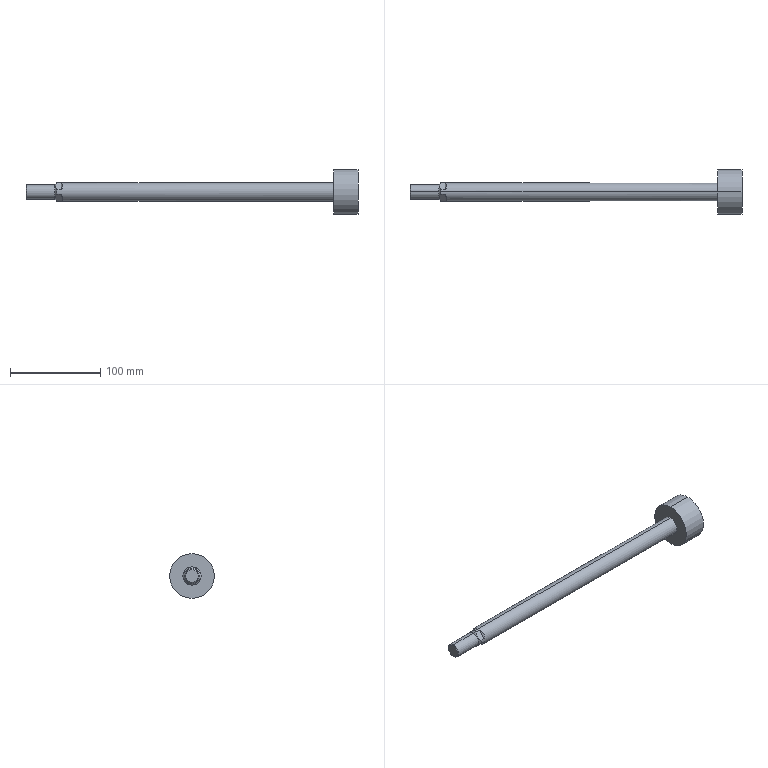Part | SolidWorks | features BaseBody 1 | 1 solid | 21 faces | box 367 x 49.5 x 49.5 mm | volume 154752 mm3 | plane 11 | cylinder 6 | cone 4 | commonest cylinder face diameters 16 x2 20 x2 49.5 x2
STEP:
#1=CARTESIAN_POINT('',(-57.,0.,-7.08));
#2=VERTEX_POINT('',#1);
#3=CARTESIAN_POINT('',(-57.,0.,7.08));
#4=VERTEX_POINT('',#3);
#5=CARTESIAN_POINT('',(-57.,0.,0.));
#6=DIRECTION('',(1.,0.,0.));
#7=DIRECTION('',(0.,0.,-1.));
#8=AXIS2_PLACEMENT_3D('',#5,#6,#7);
#9=CIRCLE('',#8,7.08);
#10=EDGE_CURVE('',#2,#4,#9,.T.);
#11=ORIENTED_EDGE('',*,*,#10,.T.);
#12=CARTESIAN_POINT('',(-56.08,0.,8.));
#13=VERTEX_POINT('',#12);
#14=CARTESIAN_POINT('',(-57.,0.,7.08));
#15=DIRECTION('',(0.7071,0.,0.7071));
#16=VECTOR('',#15,1000.);
#17=LINE('',#14,#16);
#18=EDGE_CURVE('',#4,#13,#17,.T.);
#19=ORIENTED_EDGE('',*,*,#18,.T.);
#20=CARTESIAN_POINT('',(-56.08,0.,-8.));
#21=VERTEX_POINT('',#20);
#22=CARTESIAN_POINT('',(-56.08,0.,0.));
#23=DIRECTION('',(1.,0.,0.));
#24=DIRECTION('',(0.,0.,-1.));
#25=AXIS2_PLACEMENT_3D('',#22,#23,#24);
#26=CIRCLE('',#25,8.);
#27=EDGE_CURVE('',#21,#13,#26,.T.);
#28=ORIENTED_EDGE('',*,*,#27,.F.);
#29=CARTESIAN_POINT('',(-57.,0.,-7.08));
#30=DIRECTION('',(0.7071,0.,-0.7071));
#31=VECTOR('',#30,1000.);
#32=LINE('',#29,#31);
#33=EDGE_CURVE('',#2,#21,#32,.T.);
#34=ORIENTED_EDGE('',*,*,#33,.F.);
#35=EDGE_LOOP('',(#11,#19,#28,#34));
#36=FACE_OUTER_BOUND('',#35,.T.);
#37=CARTESIAN_POINT('',(-57.,0.,0.));
#38=DIRECTION('',(1.,0.,0.));
#39=DIRECTION('',(0.,0.,-1.));
#40=AXIS2_PLACEMENT_3D('',#37,#38,#39);
#41=CONICAL_SURFACE('',#40,7.08,0.7854);
#42=ADVANCED_FACE('',(#36),#41,.T.);
#43=CARTESIAN_POINT('',(-25.,0.,8.));
#44=VERTEX_POINT('',#43);
#45=CARTESIAN_POINT('',(-25.,0.,-8.));
#46=VERTEX_POINT('',#45);
#47=CARTESIAN_POINT('',(-25.,0.,0.));
#48=DIRECTION('',(1.,0.,0.));
#49=DIRECTION('',(0.,0.,-1.));
#50=AXIS2_PLACEMENT_3D('',#47,#48,#49);
#51=CIRCLE('',#50,8.);
#52=EDGE_CURVE('',#44,#46,#51,.T.);
#53=ORIENTED_EDGE('',*,*,#52,.F.);
#54=CARTESIAN_POINT('',(310.,0.,8.));
#55=DIRECTION('',(-1.,0.,0.));
#56=VECTOR('',#55,1000.);
#57=LINE('',#54,#56);
#58=EDGE_CURVE('',#44,#13,#57,.T.);
#59=ORIENTED_EDGE('',*,*,#58,.T.);
#60=CARTESIAN_POINT('',(-56.08,0.,0.));
#61=DIRECTION('',(1.,0.,0.));
#62=DIRECTION('',(0.,0.,-1.));
#63=AXIS2_PLACEMENT_3D('',#60,#61,#62);
#64=CIRCLE('',#63,8.);
#65=EDGE_CURVE('',#13,#21,#64,.T.);
#66=ORIENTED_EDGE('',*,*,#65,.T.);
#67=CARTESIAN_POINT('',(310.,0.,-8.));
#68=DIRECTION('',(-1.,0.,0.));
#69=VECTOR('',#68,1000.);
#70=LINE('',#67,#69);
#71=EDGE_CURVE('',#46,#21,#70,.T.);
#72=ORIENTED_EDGE('',*,*,#71,.F.);
#73=EDGE_LOOP('',(#53,#59,#66,#72));
#74=FACE_OUTER_BOUND('',#73,.T.);
#75=CARTESIAN_POINT('',(310.,0.,0.));
#76=DIRECTION('',(-1.,0.,0.));
#77=DIRECTION('',(0.,0.,-1.));
#78=AXIS2_PLACEMENT_3D('',#75,#76,#77);
#79=CYLINDRICAL_SURFACE('',#78,8.);
#80=ADVANCED_FACE('',(#74),#79,.T.);
#81=CARTESIAN_POINT('',(310.,0.,24.75));
#82=VERTEX_POINT('',#81);
#83=CARTESIAN_POINT('',(310.,0.,-24.75));
#84=VERTEX_POINT('',#83);
#85=CARTESIAN_POINT('',(310.,0.,0.));
#86=DIRECTION('',(1.,0.,0.));
#87=DIRECTION('',(0.,0.,-1.));
#88=AXIS2_PLACEMENT_3D('',#85,#86,#87);
#89=CIRCLE('',#88,24.75);
#90=EDGE_CURVE('',#82,#84,#89,.T.);
#91=ORIENTED_EDGE('',*,*,#90,.F.);
#92=CARTESIAN_POINT('',(283.,0.,24.75));
#93=VERTEX_POINT('',#92);
#94=CARTESIAN_POINT('',(310.,0.,24.75));
#95=DIRECTION('',(-1.,0.,0.));
#96=VECTOR('',#95,1000.);
#97=LINE('',#94,#96);
#98=EDGE_CURVE('',#82,#93,#97,.T.);
#99=ORIENTED_EDGE('',*,*,#98,.T.);
#100=CARTESIAN_POINT('',(283.,0.,-24.75));
#101=VERTEX_POINT('',#100);
#102=CARTESIAN_POINT('',(283.,0.,0.));
#103=DIRECTION('',(1.,0.,0.));
#104=DIRECTION('',(0.,0.,-1.));
#105=AXIS2_PLACEMENT_3D('',#102,#103,#104);
#106=CIRCLE('',#105,24.75);
#107=EDGE_CURVE('',#93,#101,#106,.T.);
#108=ORIENTED_EDGE('',*,*,#107,.T.);
#109=CARTESIAN_POINT('',(310.,0.,-24.75));
#110=DIRECTION('',(-1.,0.,0.));
#111=VECTOR('',#110,1000.);
#112=LINE('',#109,#111);
#113=EDGE_CURVE('',#84,#101,#112,.T.);
#114=ORIENTED_EDGE('',*,*,#113,.F.);
#115=EDGE_LOOP('',(#91,#99,#108,#114));
#116=FACE_OUTER_BOUND('',#115,.T.);
#117=CARTESIAN_POINT('',(310.,0.,0.));
#118=DIRECTION('',(-1.,0.,0.));
#119=DIRECTION('',(0.,0.,-1.));
#120=AXIS2_PLACEMENT_3D('',#117,#118,#119);
#121=CYLINDRICAL_SURFACE('',#120,24.75);
#122=ADVANCED_FACE('',(#116),#121,.T.);
#123=CARTESIAN_POINT('',(283.,0.,10.));
#124=VERTEX_POINT('',#123);
#125=CARTESIAN_POINT('',(283.,0.,-10.));
#126=VERTEX_POINT('',#125);
#127=CARTESIAN_POINT('',(283.,0.,0.));
#128=DIRECTION('',(1.,0.,0.));
#129=DIRECTION('',(0.,0.,-1.));
#130=AXIS2_PLACEMENT_3D('',#127,#128,#129);
#131=CIRCLE('',#130,10.);
#132=EDGE_CURVE('',#124,#126,#131,.T.);
#133=ORIENTED_EDGE('',*,*,#132,.F.);
#134=CARTESIAN_POINT('',(-23.,0.,10.));
#135=VERTEX_POINT('',#134);
#136=CARTESIAN_POINT('',(310.,0.,10.));
#137=DIRECTION('',(-1.,0.,0.));
#138=VECTOR('',#137,1000.);
#139=LINE('',#136,#138);
#140=EDGE_CURVE('',#124,#135,#139,.T.);
#141=ORIENTED_EDGE('',*,*,#140,.T.);
#142=CARTESIAN_POINT('',(-23.,-2.285,9.735));
#143=VERTEX_POINT('',#142);
#144=CARTESIAN_POINT('',(-23.,0.,0.));
#145=DIRECTION('',(1.,0.,0.));
#146=DIRECTION('',(0.,0.,-1.));
#147=AXIS2_PLACEMENT_3D('',#144,#145,#146);
#148=CIRCLE('',#147,10.);
#149=EDGE_CURVE('',#135,#143,#148,.T.);
#150=ORIENTED_EDGE('',*,*,#149,.T.);
#151=CARTESIAN_POINT('',(-18.,-2.285,9.735));
#152=VERTEX_POINT('',#151);
#153=CARTESIAN_POINT('',(310.,-2.285,9.735));
#154=DIRECTION('',(-1.,0.,0.));
#155=VECTOR('',#154,1000.);
#156=LINE('',#153,#155);
#157=EDGE_CURVE('',#152,#143,#156,.T.);
#158=ORIENTED_EDGE('',*,*,#157,.F.);
#159=CARTESIAN_POINT('',(-18.,-9.735,2.285));
#160=VERTEX_POINT('',#159);
#161=CARTESIAN_POINT('',(-18.,-9.735,2.285));
#162=CARTESIAN_POINT('',(-15.944,-8.844,6.084));
#163=CARTESIAN_POINT('',(-15.944,-6.084,8.844));
#164=CARTESIAN_POINT('',(-18.,-2.285,9.735));
#165=(BOUNDED_CURVE()B_SPLINE_CURVE(3,(#161,#162,#163,#164),.UNSPECIFIED.,.F.,.F.)B_SPLINE_CURVE_WITH_KNOTS((4,4),(5.728,6.838),.UNSPECIFIED.)CURVE()GEOMETRIC_REPRESENTATION_ITEM()RATIONAL_B_SPLINE_CURVE((1.,0.9,0.9,1.))REPRESENTATION_ITEM(''));
#166=EDGE_CURVE('',#160,#152,#165,.T.);
#167=ORIENTED_EDGE('',*,*,#166,.F.);
#168=CARTESIAN_POINT('',(-23.,-9.735,2.285));
#169=VERTEX_POINT('',#168);
#170=CARTESIAN_POINT('',(310.,-9.735,2.285));
#171=DIRECTION('',(1.,0.,0.));
#172=VECTOR('',#171,1000.);
#173=LINE('',#170,#172);
#174=EDGE_CURVE('',#169,#160,#173,.T.);
#175=ORIENTED_EDGE('',*,*,#174,.F.);
#176=CARTESIAN_POINT('',(-23.,-9.735,-2.285));
#177=VERTEX_POINT('',#176);
#178=CARTESIAN_POINT('',(-23.,0.,0.));
#179=DIRECTION('',(1.,0.,0.));
#180=DIRECTION('',(0.,0.,-1.));
#181=AXIS2_PLACEMENT_3D('',#178,#179,#180);
#182=CIRCLE('',#181,10.);
#183=EDGE_CURVE('',#169,#177,#182,.T.);
#184=ORIENTED_EDGE('',*,*,#183,.T.);
#185=CARTESIAN_POINT('',(-18.,-9.735,-2.285));
#186=VERTEX_POINT('',#185);
#187=CARTESIAN_POINT('',(310.,-9.735,-2.285));
#188=DIRECTION('',(-1.,0.,0.));
#189=VECTOR('',#188,1000.);
#190=LINE('',#187,#189);
#191=EDGE_CURVE('',#186,#177,#190,.T.);
#192=ORIENTED_EDGE('',*,*,#191,.F.);
#193=CARTESIAN_POINT('',(-18.,-2.285,-9.735));
#194=VERTEX_POINT('',#193);
#195=CARTESIAN_POINT('',(-18.,-2.285,-9.735));
#196=CARTESIAN_POINT('',(-15.944,-6.084,-8.844));
#197=CARTESIAN_POINT('',(-15.944,-8.844,-6.084));
#198=CARTESIAN_POINT('',(-18.,-9.735,-2.285));
#199=(BOUNDED_CURVE()B_SPLINE_CURVE(3,(#195,#196,#197,#198),.UNSPECIFIED.,.F.,.F.)B_SPLINE_CURVE_WITH_KNOTS((4,4),(5.728,6.838),.UNSPECIFIED.)CURVE()GEOMETRIC_REPRESENTATION_ITEM()RATIONAL_B_SPLINE_CURVE((1.,0.9,0.9,1.))REPRESENTATION_ITEM(''));
#200=EDGE_CURVE('',#194,#186,#199,.T.);
#201=ORIENTED_EDGE('',*,*,#200,.F.);
#202=CARTESIAN_POINT('',(-23.,-2.285,-9.735));
#203=VERTEX_POINT('',#202);
#204=CARTESIAN_POINT('',(310.,-2.285,-9.735));
#205=DIRECTION('',(1.,0.,0.));
#206=VECTOR('',#205,1000.);
#207=LINE('',#204,#206);
#208=EDGE_CURVE('',#203,#194,#207,.T.);
#209=ORIENTED_EDGE('',*,*,#208,.F.);
#210=CARTESIAN_POINT('',(-23.,0.,-10.));
#211=VERTEX_POINT('',#210);
#212=CARTESIAN_POINT('',(-23.,0.,0.));
#213=DIRECTION('',(1.,0.,0.));
#214=DIRECTION('',(0.,0.,-1.));
#215=AXIS2_PLACEMENT_3D('',#212,#213,#214);
#216=CIRCLE('',#215,10.);
#217=EDGE_CURVE('',#203,#211,#216,.T.);
#218=ORIENTED_EDGE('',*,*,#217,.T.);
#219=CARTESIAN_POINT('',(310.,0.,-10.));
#220=DIRECTION('',(-1.,0.,0.));
#221=VECTOR('',#220,1000.);
#222=LINE('',#219,#221);
#223=EDGE_CURVE('',#126,#211,#222,.T.);
#224=ORIENTED_EDGE('',*,*,#223,.F.);
#225=EDGE_LOOP('',(#133,#141,#150,#158,#167,#175,#184,#192,#201,#209,#218,#224));
#226=FACE_OUTER_BOUND('',#225,.T.);
#227=CARTESIAN_POINT('',(310.,0.,0.));
#228=DIRECTION('',(-1.,0.,0.));
#229=DIRECTION('',(0.,0.,-1.));
#230=AXIS2_PLACEMENT_3D('',#227,#228,#229);
#231=CYLINDRICAL_SURFACE('',#230,10.);
#232=ADVANCED_FACE('',(#226),#231,.T.);
#233=CARTESIAN_POINT('',(-25.,0.,0.));
#234=DIRECTION('',(1.,0.,0.));
#235=DIRECTION('',(0.,0.,-1.));
#236=AXIS2_PLACEMENT_3D('',#233,#234,#235);
#237=CIRCLE('',#236,8.);
#238=EDGE_CURVE('',#46,#44,#237,.T.);
#239=ORIENTED_EDGE('',*,*,#238,.T.);
#240=CARTESIAN_POINT('',(-25.,0.,8.));
#241=DIRECTION('',(0.7071,0.,0.7071));
#242=VECTOR('',#241,1000.);
#243=LINE('',#240,#242);
#244=EDGE_CURVE('',#44,#135,#243,.T.);
#245=ORIENTED_EDGE('',*,*,#244,.T.);
#246=CARTESIAN_POINT('',(-23.,2.285,9.735));
#247=VERTEX_POINT('',#246);
#248=CARTESIAN_POINT('',(-23.,0.,0.));
#249=DIRECTION('',(1.,0.,0.));
#250=DIRECTION('',(0.,0.,-1.));
#251=AXIS2_PLACEMENT_3D('',#248,#249,#250);
#252=CIRCLE('',#251,10.);
#253=EDGE_CURVE('',#247,#135,#252,.T.);
#254=ORIENTED_EDGE('',*,*,#253,.F.);
#255=CARTESIAN_POINT('',(-23.,9.735,2.285));
#256=VERTEX_POINT('',#255);
#257=CARTESIAN_POINT('',(-23.,9.735,2.285));
#258=CARTESIAN_POINT('',(-23.236,9.419,2.602));
#259=CARTESIAN_POINT('',(-23.546,8.958,3.063));
#260=CARTESIAN_POINT('',(-23.834,8.441,3.58));
#261=CARTESIAN_POINT('',(-23.96,8.189,3.832));
#262=CARTESIAN_POINT('',(-24.018,8.064,3.957));
#263=CARTESIAN_POINT('',(-24.046,8.001,4.019));
#264=CARTESIAN_POINT('',(-24.057,7.975,4.046));
#265=CARTESIAN_POINT('',(-24.065,7.957,4.064));
#266=CARTESIAN_POINT('',(-24.068,7.95,4.071));
#267=CARTESIAN_POINT('',(-24.357,7.281,4.74));
#268=CARTESIAN_POINT('',(-24.5,6.638,5.383));
#269=CARTESIAN_POINT('',(-24.5,5.698,6.323));
#270=CARTESIAN_POINT('',(-24.447,5.221,6.799));
#271=CARTESIAN_POINT('',(-24.291,4.655,7.365));
#272=CARTESIAN_POINT('',(-24.19,4.37,7.651));
#273=CARTESIAN_POINT('',(-24.134,4.226,7.795));
#274=CARTESIAN_POINT('',(-24.104,4.154,7.866));
#275=CARTESIAN_POINT('',(-24.091,4.124,7.897));
#276=CARTESIAN_POINT('',(-24.082,4.103,7.918));
#277=CARTESIAN_POINT('',(-24.077,4.091,7.93));
#278=CARTESIAN_POINT('',(-23.829,3.517,8.503));
#279=CARTESIAN_POINT('',(-23.472,2.919,9.102));
#280=CARTESIAN_POINT('',(-23.,2.285,9.735));
#281=B_SPLINE_CURVE_WITH_KNOTS('',3,(#257,#258,#259,#260,#261,#262,#263,#264,#265,#266,#267,#268,#269,#270,#271,#272,#273,#274,#275,#276,#277,#278,#279,#280),.UNSPECIFIED.,.F.,.F.,(4,1,1,1,1,1,2,2,2,1,1,1,1,1,2,2,4),(0.,0.125,0.1875,0.2187,0.2344,0.2422,0.2461,0.25,0.5,0.625,0.6875,0.7188,0.7344,0.7422,0.7461,0.75,1.),.UNSPECIFIED.);
#282=EDGE_CURVE('',#256,#247,#281,.T.);
#283=ORIENTED_EDGE('',*,*,#282,.F.);
#284=CARTESIAN_POINT('',(-23.,9.735,-2.285));
#285=VERTEX_POINT('',#284);
#286=CARTESIAN_POINT('',(-23.,0.,0.));
#287=DIRECTION('',(1.,0.,0.));
#288=DIRECTION('',(0.,0.,-1.));
#289=AXIS2_PLACEMENT_3D('',#286,#287,#288);
#290=CIRCLE('',#289,10.);
#291=EDGE_CURVE('',#285,#256,#290,.T.);
#292=ORIENTED_EDGE('',*,*,#291,.F.);
#293=CARTESIAN_POINT('',(-23.,2.285,-9.735));
#294=VERTEX_POINT('',#293);
#295=CARTESIAN_POINT('',(-23.,2.285,-9.735));
#296=CARTESIAN_POINT('',(-23.236,2.602,-9.419));
#297=CARTESIAN_POINT('',(-23.546,3.063,-8.958));
#298=CARTESIAN_POINT('',(-23.834,3.58,-8.441));
#299=CARTESIAN_POINT('',(-23.96,3.832,-8.189));
#300=CARTESIAN_POINT('',(-24.018,3.957,-8.064));
#301=CARTESIAN_POINT('',(-24.046,4.019,-8.001));
#302=CARTESIAN_POINT('',(-24.057,4.046,-7.975));
#303=CARTESIAN_POINT('',(-24.065,4.064,-7.957));
#304=CARTESIAN_POINT('',(-24.068,4.071,-7.95));
#305=CARTESIAN_POINT('',(-24.357,4.74,-7.281));
#306=CARTESIAN_POINT('',(-24.5,5.383,-6.638));
#307=CARTESIAN_POINT('',(-24.5,6.323,-5.698));
#308=CARTESIAN_POINT('',(-24.447,6.799,-5.221));
#309=CARTESIAN_POINT('',(-24.291,7.365,-4.655));
#310=CARTESIAN_POINT('',(-24.19,7.651,-4.37));
#311=CARTESIAN_POINT('',(-24.134,7.795,-4.226));
#312=CARTESIAN_POINT('',(-24.104,7.866,-4.154));
#313=CARTESIAN_POINT('',(-24.091,7.897,-4.124));
#314=CARTESIAN_POINT('',(-24.082,7.918,-4.103));
#315=CARTESIAN_POINT('',(-24.077,7.93,-4.091));
#316=CARTESIAN_POINT('',(-23.829,8.503,-3.517));
#317=CARTESIAN_POINT('',(-23.472,9.102,-2.919));
#318=CARTESIAN_POINT('',(-23.,9.735,-2.285));
#319=B_SPLINE_CURVE_WITH_KNOTS('',3,(#295,#296,#297,#298,#299,#300,#301,#302,#303,#304,#305,#306,#307,#308,#309,#310,#311,#312,#313,#314,#315,#316,#317,#318),.UNSPECIFIED.,.F.,.F.,(4,1,1,1,1,1,2,2,2,1,1,1,1,1,2,2,4),(0.,0.125,0.1875,0.2188,0.2344,0.2422,0.2461,0.25,0.5,0.625,0.6875,0.7188,0.7344,0.7422,0.7461,0.75,1.),.UNSPECIFIED.);
#320=EDGE_CURVE('',#294,#285,#319,.T.);
#321=ORIENTED_EDGE('',*,*,#320,.F.);
#322=CARTESIAN_POINT('',(-23.,0.,0.));
#323=DIRECTION('',(1.,0.,0.));
#324=DIRECTION('',(0.,0.,-1.));
#325=AXIS2_PLACEMENT_3D('',#322,#323,#324);
#326=CIRCLE('',#325,10.);
#327=EDGE_CURVE('',#211,#294,#326,.T.);
#328=ORIENTED_EDGE('',*,*,#327,.F.);
#329=CARTESIAN_POINT('',(-25.,0.,-8.));
#330=DIRECTION('',(0.7071,0.,-0.7071));
#331=VECTOR('',#330,1000.);
#332=LINE('',#329,#331);
#333=EDGE_CURVE('',#46,#211,#332,.T.);
#334=ORIENTED_EDGE('',*,*,#333,.F.);
#335=EDGE_LOOP('',(#239,#245,#254,#283,#292,#321,#328,#334));
#336=FACE_OUTER_BOUND('',#335,.T.);
#337=CARTESIAN_POINT('',(-25.,0.,0.));
#338=DIRECTION('',(1.,0.,0.));
#339=DIRECTION('',(0.,0.,-1.));
#340=AXIS2_PLACEMENT_3D('',#337,#338,#339);
#341=CONICAL_SURFACE('',#340,8.,0.7854);
#342=ADVANCED_FACE('',(#336),#341,.T.);
#343=CARTESIAN_POINT('',(-18.,9.735,-2.285));
#344=VERTEX_POINT('',#343);
#345=CARTESIAN_POINT('',(310.,9.735,-2.285));
#346=DIRECTION('',(1.,0.,0.));
#347=VECTOR('',#346,1000.);
#348=LINE('',#345,#347);
#349=EDGE_CURVE('',#285,#344,#348,.T.);
#350=ORIENTED_EDGE('',*,*,#349,.T.);
#351=CARTESIAN_POINT('',(-18.,2.285,-9.735));
#352=VERTEX_POINT('',#351);
#353=CARTESIAN_POINT('',(-18.,-6.01,-18.031));
#354=DIRECTION('',(0.,0.7071,0.7071));
#355=VECTOR('',#354,1000.);
#356=LINE('',#353,#355);
#357=EDGE_CURVE('',#352,#344,#356,.T.);
#358=ORIENTED_EDGE('',*,*,#357,.F.);
#359=CARTESIAN_POINT('',(310.,2.285,-9.735));
#360=DIRECTION('',(-1.,0.,0.));
#361=VECTOR('',#360,1000.);
#362=LINE('',#359,#361);
#363=EDGE_CURVE('',#352,#294,#362,.T.);
#364=ORIENTED_EDGE('',*,*,#363,.T.);
#365=ORIENTED_EDGE('',*,*,#320,.T.);
#366=EDGE_LOOP('',(#350,#358,#364,#365));
#367=FACE_OUTER_BOUND('',#366,.T.);
#368=CARTESIAN_POINT('',(-18.,-6.01,-18.031));
#369=DIRECTION('',(0.,0.7071,-0.7071));
#370=DIRECTION('',(-1.,0.,0.));
#371=AXIS2_PLACEMENT_3D('',#368,#369,#370);
#372=PLANE('',#371);
#373=ADVANCED_FACE('',(#367),#372,.T.);
#374=CARTESIAN_POINT('',(-18.,9.735,-2.285));
#375=CARTESIAN_POINT('',(-15.944,8.844,-6.084));
#376=CARTESIAN_POINT('',(-15.944,6.084,-8.844));
#377=CARTESIAN_POINT('',(-18.,2.285,-9.735));
#378=(BOUNDED_CURVE()B_SPLINE_CURVE(3,(#374,#375,#376,#377),.UNSPECIFIED.,.F.,.F.)B_SPLINE_CURVE_WITH_KNOTS((4,4),(5.728,6.838),.UNSPECIFIED.)CURVE()GEOMETRIC_REPRESENTATION_ITEM()RATIONAL_B_SPLINE_CURVE((1.,0.9,0.9,1.))REPRESENTATION_ITEM(''));
#379=EDGE_CURVE('',#344,#352,#378,.T.);
#380=ORIENTED_EDGE('',*,*,#379,.T.);
#381=ORIENTED_EDGE('',*,*,#357,.T.);
#382=EDGE_LOOP('',(#380,#381));
#383=FACE_OUTER_BOUND('',#382,.T.);
#384=CARTESIAN_POINT('',(-1.,6.01,-30.052));
#385=DIRECTION('',(-0.7071,0.5,-0.5));
#386=DIRECTION('',(-0.5774,0.,0.8165));
#387=AXIS2_PLACEMENT_3D('',#384,#385,#386);
#388=PLANE('',#387);
#389=ADVANCED_FACE('',(#383),#388,.T.);
#390=CARTESIAN_POINT('',(-18.,2.285,9.735));
#391=VERTEX_POINT('',#390);
#392=CARTESIAN_POINT('',(-18.,9.735,2.285));
#393=VERTEX_POINT('',#392);
#394=CARTESIAN_POINT('',(-18.,2.285,9.735));
#395=CARTESIAN_POINT('',(-15.944,6.084,8.844));
#396=CARTESIAN_POINT('',(-15.944,8.844,6.084));
#397=CARTESIAN_POINT('',(-18.,9.735,2.285));
#398=(BOUNDED_CURVE()B_SPLINE_CURVE(3,(#394,#395,#396,#397),.UNSPECIFIED.,.F.,.F.)B_SPLINE_CURVE_WITH_KNOTS((4,4),(5.728,6.838),.UNSPECIFIED.)CURVE()GEOMETRIC_REPRESENTATION_ITEM()RATIONAL_B_SPLINE_CURVE((1.,0.9,0.9,1.))REPRESENTATION_ITEM(''));
#399=EDGE_CURVE('',#391,#393,#398,.T.);
#400=ORIENTED_EDGE('',*,*,#399,.T.);
#401=CARTESIAN_POINT('',(-18.,-6.01,18.031));
#402=DIRECTION('',(0.,0.7071,-0.7071));
#403=VECTOR('',#402,1000.);
#404=LINE('',#401,#403);
#405=EDGE_CURVE('',#391,#393,#404,.T.);
#406=ORIENTED_EDGE('',*,*,#405,.F.);
#407=EDGE_LOOP('',(#400,#406));
#408=FACE_OUTER_BOUND('',#407,.T.);
#409=CARTESIAN_POINT('',(-18.,-6.01,18.031));
#410=DIRECTION('',(-0.7071,0.5,0.5));
#411=DIRECTION('',(0.5774,0.,0.8165));
#412=AXIS2_PLACEMENT_3D('',#409,#410,#411);
#413=PLANE('',#412);
#414=ADVANCED_FACE('',(#408),#413,.T.);
#415=CARTESIAN_POINT('',(310.,2.285,9.735));
#416=DIRECTION('',(1.,0.,0.));
#417=VECTOR('',#416,1000.);
#418=LINE('',#415,#417);
#419=EDGE_CURVE('',#247,#391,#418,.T.);
#420=ORIENTED_EDGE('',*,*,#419,.T.);
#421=ORIENTED_EDGE('',*,*,#405,.T.);
#422=CARTESIAN_POINT('',(310.,9.735,2.285));
#423=DIRECTION('',(-1.,0.,0.));
#424=VECTOR('',#423,1000.);
#425=LINE('',#422,#424);
#426=EDGE_CURVE('',#393,#256,#425,.T.);
#427=ORIENTED_EDGE('',*,*,#426,.T.);
#428=ORIENTED_EDGE('',*,*,#282,.T.);
#429=EDGE_LOOP('',(#420,#421,#427,#428));
#430=FACE_OUTER_BOUND('',#429,.T.);
#431=CARTESIAN_POINT('',(-57.,-6.01,18.031));
#432=DIRECTION('',(0.,0.7071,0.7071));
#433=DIRECTION('',(1.,0.,0.));
#434=AXIS2_PLACEMENT_3D('',#431,#432,#433);
#435=PLANE('',#434);
#436=ADVANCED_FACE('',(#430),#435,.T.);
#437=ORIENTED_EDGE('',*,*,#200,.T.);
#438=CARTESIAN_POINT('',(-18.,-18.031,6.01));
#439=DIRECTION('',(0.,0.7071,-0.7071));
#440=VECTOR('',#439,1000.);
#441=LINE('',#438,#440);
#442=EDGE_CURVE('',#186,#194,#441,.T.);
#443=ORIENTED_EDGE('',*,*,#442,.T.);
#444=EDGE_LOOP('',(#437,#443));
#445=FACE_OUTER_BOUND('',#444,.T.);
#446=CARTESIAN_POINT('',(-1.,-30.052,-6.01));
#447=DIRECTION('',(-0.7071,-0.5,-0.5));
#448=DIRECTION('',(-0.5774,0.,0.8165));
#449=AXIS2_PLACEMENT_3D('',#446,#447,#448);
#450=PLANE('',#449);
#451=ADVANCED_FACE('',(#445),#450,.T.);
#452=ORIENTED_EDGE('',*,*,#208,.T.);
#453=ORIENTED_EDGE('',*,*,#442,.F.);
#454=ORIENTED_EDGE('',*,*,#191,.T.);
#455=CARTESIAN_POINT('',(-23.,-9.735,-2.285));
#456=CARTESIAN_POINT('',(-23.236,-9.419,-2.602));
#457=CARTESIAN_POINT('',(-23.546,-8.958,-3.063));
#458=CARTESIAN_POINT('',(-23.834,-8.441,-3.58));
#459=CARTESIAN_POINT('',(-23.96,-8.189,-3.832));
#460=CARTESIAN_POINT('',(-24.018,-8.064,-3.957));
#461=CARTESIAN_POINT('',(-24.046,-8.001,-4.019));
#462=CARTESIAN_POINT('',(-24.057,-7.975,-4.046));
#463=CARTESIAN_POINT('',(-24.065,-7.957,-4.064));
#464=CARTESIAN_POINT('',(-24.068,-7.95,-4.071));
#465=CARTESIAN_POINT('',(-24.357,-7.281,-4.74));
#466=CARTESIAN_POINT('',(-24.5,-6.638,-5.383));
#467=CARTESIAN_POINT('',(-24.5,-5.698,-6.323));
#468=CARTESIAN_POINT('',(-24.447,-5.221,-6.799));
#469=CARTESIAN_POINT('',(-24.291,-4.655,-7.365));
#470=CARTESIAN_POINT('',(-24.19,-4.37,-7.651));
#471=CARTESIAN_POINT('',(-24.134,-4.226,-7.795));
#472=CARTESIAN_POINT('',(-24.104,-4.154,-7.866));
#473=CARTESIAN_POINT('',(-24.091,-4.124,-7.897));
#474=CARTESIAN_POINT('',(-24.082,-4.103,-7.918));
#475=CARTESIAN_POINT('',(-24.077,-4.091,-7.93));
#476=CARTESIAN_POINT('',(-23.829,-3.517,-8.503));
#477=CARTESIAN_POINT('',(-23.472,-2.919,-9.102));
#478=CARTESIAN_POINT('',(-23.,-2.285,-9.735));
#479=B_SPLINE_CURVE_WITH_KNOTS('',3,(#455,#456,#457,#458,#459,#460,#461,#462,#463,#464,#465,#466,#467,#468,#469,#470,#471,#472,#473,#474,#475,#476,#477,#478),.UNSPECIFIED.,.F.,.F.,(4,1,1,1,1,1,2,2,2,1,1,1,1,1,2,2,4),(0.,0.125,0.1875,0.2187,0.2344,0.2422,0.2461,0.25,0.5,0.625,0.6875,0.7188,0.7344,0.7422,0.7461,0.75,1.),.UNSPECIFIED.);
#480=EDGE_CURVE('',#177,#203,#479,.T.);
#481=ORIENTED_EDGE('',*,*,#480,.T.);
#482=EDGE_LOOP('',(#452,#453,#454,#481));
#483=FACE_OUTER_BOUND('',#482,.T.);
#484=CARTESIAN_POINT('',(-18.,-18.031,6.01));
#485=DIRECTION('',(0.,-0.7071,-0.7071));
#486=DIRECTION('',(0.,-0.7071,0.7071));
#487=AXIS2_PLACEMENT_3D('',#484,#485,#486);
#488=PLANE('',#487);
#489=ADVANCED_FACE('',(#483),#488,.T.);
#490=ORIENTED_EDGE('',*,*,#244,.F.);
#491=ORIENTED_EDGE('',*,*,#52,.T.);
#492=ORIENTED_EDGE('',*,*,#333,.T.);
#493=ORIENTED_EDGE('',*,*,#217,.F.);
#494=ORIENTED_EDGE('',*,*,#480,.F.);
#495=ORIENTED_EDGE('',*,*,#183,.F.);
#496=CARTESIAN_POINT('',(-23.,-2.285,9.735));
#497=CARTESIAN_POINT('',(-23.236,-2.602,9.419));
#498=CARTESIAN_POINT('',(-23.546,-3.063,8.958));
#499=CARTESIAN_POINT('',(-23.834,-3.58,8.441));
#500=CARTESIAN_POINT('',(-23.96,-3.832,8.189));
#501=CARTESIAN_POINT('',(-24.018,-3.957,8.064));
#502=CARTESIAN_POINT('',(-24.046,-4.019,8.001));
#503=CARTESIAN_POINT('',(-24.057,-4.046,7.975));
#504=CARTESIAN_POINT('',(-24.065,-4.064,7.957));
#505=CARTESIAN_POINT('',(-24.068,-4.071,7.95));
#506=CARTESIAN_POINT('',(-24.357,-4.74,7.281));
#507=CARTESIAN_POINT('',(-24.5,-5.383,6.638));
#508=CARTESIAN_POINT('',(-24.5,-6.323,5.698));
#509=CARTESIAN_POINT('',(-24.447,-6.799,5.221));
#510=CARTESIAN_POINT('',(-24.291,-7.365,4.655));
#511=CARTESIAN_POINT('',(-24.19,-7.651,4.37));
#512=CARTESIAN_POINT('',(-24.134,-7.795,4.226));
#513=CARTESIAN_POINT('',(-24.104,-7.866,4.154));
#514=CARTESIAN_POINT('',(-24.091,-7.897,4.124));
#515=CARTESIAN_POINT('',(-24.082,-7.918,4.103));
#516=CARTESIAN_POINT('',(-24.077,-7.93,4.091));
#517=CARTESIAN_POINT('',(-23.829,-8.503,3.517));
#518=CARTESIAN_POINT('',(-23.472,-9.102,2.919));
#519=CARTESIAN_POINT('',(-23.,-9.735,2.285));
#520=B_SPLINE_CURVE_WITH_KNOTS('',3,(#496,#497,#498,#499,#500,#501,#502,#503,#504,#505,#506,#507,#508,#509,#510,#511,#512,#513,#514,#515,#516,#517,#518,#519),.UNSPECIFIED.,.F.,.F.,(4,1,1,1,1,1,2,2,2,1,1,1,1,1,2,2,4),(0.,0.125,0.1875,0.2187,0.2344,0.2422,0.2461,0.25,0.5,0.625,0.6875,0.7188,0.7344,0.7422,0.7461,0.75,1.),.UNSPECIFIED.);
#521=EDGE_CURVE('',#143,#169,#520,.T.);
#522=ORIENTED_EDGE('',*,*,#521,.F.);
#523=ORIENTED_EDGE('',*,*,#149,.F.);
#524=EDGE_LOOP('',(#490,#491,#492,#493,#494,#495,#522,#523));
#525=FACE_OUTER_BOUND('',#524,.T.);
#526=CARTESIAN_POINT('',(-25.,0.,0.));
#527=DIRECTION('',(1.,0.,0.));
#528=DIRECTION('',(0.,0.,-1.));
#529=AXIS2_PLACEMENT_3D('',#526,#527,#528);
#530=CONICAL_SURFACE('',#529,8.,0.7854);
#531=ADVANCED_FACE('',(#525),#530,.T.);
#532=ORIENTED_EDGE('',*,*,#140,.F.);
#533=CARTESIAN_POINT('',(283.,0.,0.));
#534=DIRECTION('',(1.,0.,0.));
#535=DIRECTION('',(0.,0.,-1.));
#536=AXIS2_PLACEMENT_3D('',#533,#534,#535);
#537=CIRCLE('',#536,10.);
#538=EDGE_CURVE('',#126,#124,#537,.T.);
#539=ORIENTED_EDGE('',*,*,#538,.F.);
#540=ORIENTED_EDGE('',*,*,#223,.T.);
#541=ORIENTED_EDGE('',*,*,#327,.T.);
#542=ORIENTED_EDGE('',*,*,#363,.F.);
#543=ORIENTED_EDGE('',*,*,#379,.F.);
#544=ORIENTED_EDGE('',*,*,#349,.F.);
#545=ORIENTED_EDGE('',*,*,#291,.T.);
#546=ORIENTED_EDGE('',*,*,#426,.F.);
#547=ORIENTED_EDGE('',*,*,#399,.F.);
#548=ORIENTED_EDGE('',*,*,#419,.F.);
#549=ORIENTED_EDGE('',*,*,#253,.T.);
#550=EDGE_LOOP('',(#532,#539,#540,#541,#542,#543,#544,#545,#546,#547,#548,#549));
#551=FACE_OUTER_BOUND('',#550,.T.);
#552=CARTESIAN_POINT('',(310.,0.,0.));
#553=DIRECTION('',(-1.,0.,0.));
#554=DIRECTION('',(0.,0.,-1.));
#555=AXIS2_PLACEMENT_3D('',#552,#553,#554);
#556=CYLINDRICAL_SURFACE('',#555,10.);
#557=ADVANCED_FACE('',(#551),#556,.T.);
#558=ORIENTED_EDGE('',*,*,#10,.F.);
#559=CARTESIAN_POINT('',(-57.,0.,0.));
#560=DIRECTION('',(1.,0.,0.));
#561=DIRECTION('',(0.,0.,-1.));
#562=AXIS2_PLACEMENT_3D('',#559,#560,#561);
#563=CIRCLE('',#562,7.08);
#564=EDGE_CURVE('',#4,#2,#563,.T.);
#565=ORIENTED_EDGE('',*,*,#564,.F.);
#566=EDGE_LOOP('',(#558,#565));
#567=FACE_OUTER_BOUND('',#566,.T.);
#568=CARTESIAN_POINT('',(-57.,0.,0.));
#569=DIRECTION('',(1.,0.,0.));
#570=DIRECTION('',(0.,1.,0.));
#571=AXIS2_PLACEMENT_3D('',#568,#569,#570);
#572=PLANE('',#571);
#573=ADVANCED_FACE('',(#567),#572,.F.);
#574=CARTESIAN_POINT('',(283.,0.,0.));
#575=DIRECTION('',(1.,0.,0.));
#576=DIRECTION('',(0.,0.,-1.));
#577=AXIS2_PLACEMENT_3D('',#574,#575,#576);
#578=CIRCLE('',#577,24.75);
#579=EDGE_CURVE('',#101,#93,#578,.T.);
#580=ORIENTED_EDGE('',*,*,#579,.F.);
#581=ORIENTED_EDGE('',*,*,#107,.F.);
#582=EDGE_LOOP('',(#580,#581));
#583=FACE_OUTER_BOUND('',#582,.T.);
#584=ORIENTED_EDGE('',*,*,#538,.T.);
#585=ORIENTED_EDGE('',*,*,#132,.T.);
#586=EDGE_LOOP('',(#584,#585));
#587=FACE_BOUND('',#586,.T.);
#588=CARTESIAN_POINT('',(283.,10.,0.));
#589=DIRECTION('',(1.,0.,0.));
#590=DIRECTION('',(0.,1.,0.));
#591=AXIS2_PLACEMENT_3D('',#588,#589,#590);
#592=PLANE('',#591);
#593=ADVANCED_FACE('',(#583,#587),#592,.F.);
#594=ORIENTED_EDGE('',*,*,#98,.F.);
#595=CARTESIAN_POINT('',(310.,0.,0.));
#596=DIRECTION('',(1.,0.,0.));
#597=DIRECTION('',(0.,0.,-1.));
#598=AXIS2_PLACEMENT_3D('',#595,#596,#597);
#599=CIRCLE('',#598,24.75);
#600=EDGE_CURVE('',#84,#82,#599,.T.);
#601=ORIENTED_EDGE('',*,*,#600,.F.);
#602=ORIENTED_EDGE('',*,*,#113,.T.);
#603=ORIENTED_EDGE('',*,*,#579,.T.);
#604=EDGE_LOOP('',(#594,#601,#602,#603));
#605=FACE_OUTER_BOUND('',#604,.T.);
#606=CARTESIAN_POINT('',(310.,0.,0.));
#607=DIRECTION('',(-1.,0.,0.));
#608=DIRECTION('',(0.,0.,-1.));
#609=AXIS2_PLACEMENT_3D('',#606,#607,#608);
#610=CYLINDRICAL_SURFACE('',#609,24.75);
#611=ADVANCED_FACE('',(#605),#610,.T.);
#612=ORIENTED_EDGE('',*,*,#600,.T.);
#613=ORIENTED_EDGE('',*,*,#90,.T.);
#614=EDGE_LOOP('',(#612,#613));
#615=FACE_OUTER_BOUND('',#614,.T.);
#616=CARTESIAN_POINT('',(310.,24.75,0.));
#617=DIRECTION('',(-1.,0.,0.));
#618=DIRECTION('',(0.,0.,1.));
#619=AXIS2_PLACEMENT_3D('',#616,#617,#618);
#620=PLANE('',#619);
#621=ADVANCED_FACE('',(#615),#620,.F.);
#622=ORIENTED_EDGE('',*,*,#58,.F.);
#623=ORIENTED_EDGE('',*,*,#238,.F.);
#624=ORIENTED_EDGE('',*,*,#71,.T.);
#625=ORIENTED_EDGE('',*,*,#27,.T.);
#626=EDGE_LOOP('',(#622,#623,#624,#625));
#627=FACE_OUTER_BOUND('',#626,.T.);
#628=CARTESIAN_POINT('',(310.,0.,0.));
#629=DIRECTION('',(-1.,0.,0.));
#630=DIRECTION('',(0.,0.,-1.));
#631=AXIS2_PLACEMENT_3D('',#628,#629,#630);
#632=CYLINDRICAL_SURFACE('',#631,8.);
#633=ADVANCED_FACE('',(#627),#632,.T.);
#634=ORIENTED_EDGE('',*,*,#18,.F.);
#635=ORIENTED_EDGE('',*,*,#564,.T.);
#636=ORIENTED_EDGE('',*,*,#33,.T.);
#637=ORIENTED_EDGE('',*,*,#65,.F.);
#638=EDGE_LOOP('',(#634,#635,#636,#637));
#639=FACE_OUTER_BOUND('',#638,.T.);
#640=CARTESIAN_POINT('',(-57.,0.,0.));
#641=DIRECTION('',(1.,0.,0.));
#642=DIRECTION('',(0.,0.,-1.));
#643=AXIS2_PLACEMENT_3D('',#640,#641,#642);
#644=CONICAL_SURFACE('',#643,7.08,0.7854);
#645=ADVANCED_FACE('',(#639),#644,.T.);
#646=ORIENTED_EDGE('',*,*,#166,.T.);
#647=CARTESIAN_POINT('',(-18.,-18.031,-6.01));
#648=DIRECTION('',(0.,0.7071,0.7071));
#649=VECTOR('',#648,1000.);
#650=LINE('',#647,#649);
#651=EDGE_CURVE('',#160,#152,#650,.T.);
#652=ORIENTED_EDGE('',*,*,#651,.F.);
#653=EDGE_LOOP('',(#646,#652));
#654=FACE_OUTER_BOUND('',#653,.T.);
#655=CARTESIAN_POINT('',(-18.,-18.031,-6.01));
#656=DIRECTION('',(-0.7071,-0.5,0.5));
#657=DIRECTION('',(-0.5774,0.8165,0.));
#658=AXIS2_PLACEMENT_3D('',#655,#656,#657);
#659=PLANE('',#658);
#660=ADVANCED_FACE('',(#654),#659,.T.);
#661=ORIENTED_EDGE('',*,*,#174,.T.);
#662=ORIENTED_EDGE('',*,*,#651,.T.);
#663=ORIENTED_EDGE('',*,*,#157,.T.);
#664=ORIENTED_EDGE('',*,*,#521,.T.);
#665=EDGE_LOOP('',(#661,#662,#663,#664));
#666=FACE_OUTER_BOUND('',#665,.T.);
#667=CARTESIAN_POINT('',(-57.,-18.031,-6.01));
#668=DIRECTION('',(0.,-0.7071,0.7071));
#669=DIRECTION('',(-1.,0.,0.));
#670=AXIS2_PLACEMENT_3D('',#667,#668,#669);
#671=PLANE('',#670);
#672=ADVANCED_FACE('',(#666),#671,.T.);
#673=CLOSED_SHELL('',(#42,#80,#122,#232,#342,#373,#389,#414,#436,#451,#489,#531,#557,#573,#593,#611,#621,#633,#645,#660,#672));
#674=MANIFOLD_SOLID_BREP('',#673);
#675=CARTESIAN_POINT('',(0.,0.,0.));
#676=DIRECTION('',(0.,0.,1.));
#677=DIRECTION('',(1.,0.,0.));
#678=AXIS2_PLACEMENT_3D('',#675,#676,#677);
#679=(LENGTH_UNIT()NAMED_UNIT(*)SI_UNIT(.MILLI.,.METRE.));
#680=UNCERTAINTY_MEASURE_WITH_UNIT(LENGTH_MEASURE(0.00001),#679,'','');
#681=(NAMED_UNIT(*)PLANE_ANGLE_UNIT()SI_UNIT($,.RADIAN.));
#682=(NAMED_UNIT(*)SI_UNIT($,.STERADIAN.)SOLID_ANGLE_UNIT());
#683=(GEOMETRIC_REPRESENTATION_CONTEXT(3)GLOBAL_UNCERTAINTY_ASSIGNED_CONTEXT((#680))GLOBAL_UNIT_ASSIGNED_CONTEXT((#679,#681,#682))REPRESENTATION_CONTEXT('',''));
#684=ADVANCED_BREP_SHAPE_REPRESENTATION('',(#674,#678),#683);